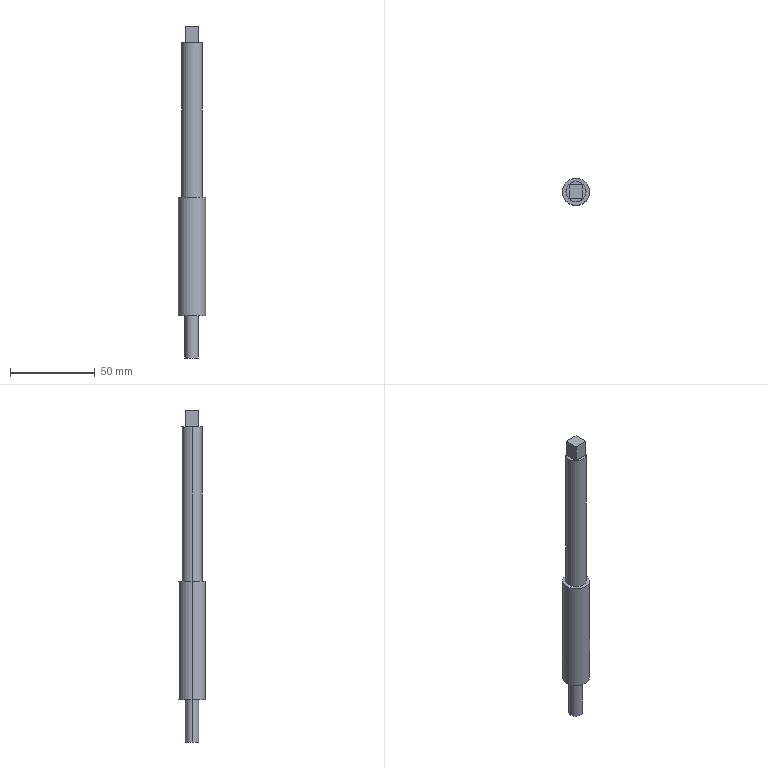Part | SolidWorks | features ICE 3, Extrusion 1 | 1 solid | 15 faces | box 16 x 16 x 196 mm | volume 26092 mm3 | plane 9 | cylinder 6 | commonest cylinder face diameters 8 x2 11.9 x2 16 x2
STEP:
#1=CARTESIAN_POINT('',(-4.225,0.,-95.));
#2=VERTEX_POINT('',#1);
#3=CARTESIAN_POINT('',(3.775,0.,-95.));
#4=VERTEX_POINT('',#3);
#5=CARTESIAN_POINT('',(-0.2246,0.,-95.));
#6=DIRECTION('',(0.,0.,-1.));
#7=DIRECTION('',(-1.,0.,0.));
#8=AXIS2_PLACEMENT_3D('',#5,#6,#7);
#9=CIRCLE('',#8,4.);
#10=EDGE_CURVE('',#2,#4,#9,.T.);
#11=ORIENTED_EDGE('',*,*,#10,.F.);
#12=CARTESIAN_POINT('',(-4.225,0.,-70.));
#13=VERTEX_POINT('',#12);
#14=CARTESIAN_POINT('',(-4.225,0.,-95.));
#15=DIRECTION('',(0.,0.,1.));
#16=VECTOR('',#15,1000.);
#17=LINE('',#14,#16);
#18=EDGE_CURVE('',#2,#13,#17,.T.);
#19=ORIENTED_EDGE('',*,*,#18,.T.);
#20=CARTESIAN_POINT('',(3.775,0.,-70.));
#21=VERTEX_POINT('',#20);
#22=CARTESIAN_POINT('',(-0.2246,0.,-70.));
#23=DIRECTION('',(0.,0.,-1.));
#24=DIRECTION('',(-1.,0.,0.));
#25=AXIS2_PLACEMENT_3D('',#22,#23,#24);
#26=CIRCLE('',#25,4.);
#27=EDGE_CURVE('',#13,#21,#26,.T.);
#28=ORIENTED_EDGE('',*,*,#27,.T.);
#29=CARTESIAN_POINT('',(3.775,0.,-95.));
#30=DIRECTION('',(0.,0.,1.));
#31=VECTOR('',#30,1000.);
#32=LINE('',#29,#31);
#33=EDGE_CURVE('',#4,#21,#32,.T.);
#34=ORIENTED_EDGE('',*,*,#33,.F.);
#35=EDGE_LOOP('',(#11,#19,#28,#34));
#36=FACE_OUTER_BOUND('',#35,.T.);
#37=CARTESIAN_POINT('',(-0.2246,0.,-95.));
#38=DIRECTION('',(0.,0.,1.));
#39=DIRECTION('',(1.,0.,0.));
#40=AXIS2_PLACEMENT_3D('',#37,#38,#39);
#41=CYLINDRICAL_SURFACE('',#40,4.);
#42=ADVANCED_FACE('',(#36),#41,.T.);
#43=CARTESIAN_POINT('',(-8.,0.,-70.));
#44=VERTEX_POINT('',#43);
#45=CARTESIAN_POINT('',(8.,0.,-70.));
#46=VERTEX_POINT('',#45);
#47=CARTESIAN_POINT('',(0.,0.,-70.));
#48=DIRECTION('',(0.,0.,-1.));
#49=DIRECTION('',(-1.,0.,0.));
#50=AXIS2_PLACEMENT_3D('',#47,#48,#49);
#51=CIRCLE('',#50,8.);
#52=EDGE_CURVE('',#44,#46,#51,.T.);
#53=ORIENTED_EDGE('',*,*,#52,.F.);
#54=CARTESIAN_POINT('',(-8.,0.,0.));
#55=VERTEX_POINT('',#54);
#56=CARTESIAN_POINT('',(-8.,0.,-70.));
#57=DIRECTION('',(0.,0.,1.));
#58=VECTOR('',#57,1000.);
#59=LINE('',#56,#58);
#60=EDGE_CURVE('',#44,#55,#59,.T.);
#61=ORIENTED_EDGE('',*,*,#60,.T.);
#62=CARTESIAN_POINT('',(8.,0.,0.));
#63=VERTEX_POINT('',#62);
#64=CARTESIAN_POINT('',(0.,0.,0.));
#65=DIRECTION('',(0.,0.,-1.));
#66=DIRECTION('',(-1.,0.,0.));
#67=AXIS2_PLACEMENT_3D('',#64,#65,#66);
#68=CIRCLE('',#67,8.);
#69=EDGE_CURVE('',#55,#63,#68,.T.);
#70=ORIENTED_EDGE('',*,*,#69,.T.);
#71=CARTESIAN_POINT('',(8.,0.,-70.));
#72=DIRECTION('',(0.,0.,1.));
#73=VECTOR('',#72,1000.);
#74=LINE('',#71,#73);
#75=EDGE_CURVE('',#46,#63,#74,.T.);
#76=ORIENTED_EDGE('',*,*,#75,.F.);
#77=EDGE_LOOP('',(#53,#61,#70,#76));
#78=FACE_OUTER_BOUND('',#77,.T.);
#79=CARTESIAN_POINT('',(0.,0.,-70.));
#80=DIRECTION('',(0.,0.,1.));
#81=DIRECTION('',(1.,0.,0.));
#82=AXIS2_PLACEMENT_3D('',#79,#80,#81);
#83=CYLINDRICAL_SURFACE('',#82,8.);
#84=ADVANCED_FACE('',(#78),#83,.T.);
#85=CARTESIAN_POINT('',(5.95,0.,91.));
#86=VERTEX_POINT('',#85);
#87=CARTESIAN_POINT('',(-5.95,0.,91.));
#88=VERTEX_POINT('',#87);
#89=CARTESIAN_POINT('',(0.,0.,91.));
#90=DIRECTION('',(0.,0.,1.));
#91=DIRECTION('',(1.,0.,0.));
#92=AXIS2_PLACEMENT_3D('',#89,#90,#91);
#93=CIRCLE('',#92,5.95);
#94=EDGE_CURVE('',#86,#88,#93,.T.);
#95=ORIENTED_EDGE('',*,*,#94,.F.);
#96=CARTESIAN_POINT('',(5.95,0.,0.));
#97=VERTEX_POINT('',#96);
#98=CARTESIAN_POINT('',(5.95,0.,91.));
#99=DIRECTION('',(0.,0.,-1.));
#100=VECTOR('',#99,1000.);
#101=LINE('',#98,#100);
#102=EDGE_CURVE('',#86,#97,#101,.T.);
#103=ORIENTED_EDGE('',*,*,#102,.T.);
#104=CARTESIAN_POINT('',(-5.95,0.,0.));
#105=VERTEX_POINT('',#104);
#106=CARTESIAN_POINT('',(0.,0.,0.));
#107=DIRECTION('',(0.,0.,-1.));
#108=DIRECTION('',(-1.,0.,0.));
#109=AXIS2_PLACEMENT_3D('',#106,#107,#108);
#110=CIRCLE('',#109,5.95);
#111=EDGE_CURVE('',#105,#97,#110,.T.);
#112=ORIENTED_EDGE('',*,*,#111,.F.);
#113=CARTESIAN_POINT('',(-5.95,0.,91.));
#114=DIRECTION('',(0.,0.,-1.));
#115=VECTOR('',#114,1000.);
#116=LINE('',#113,#115);
#117=EDGE_CURVE('',#88,#105,#116,.T.);
#118=ORIENTED_EDGE('',*,*,#117,.F.);
#119=EDGE_LOOP('',(#95,#103,#112,#118));
#120=FACE_OUTER_BOUND('',#119,.T.);
#121=CARTESIAN_POINT('',(0.,0.,91.));
#122=DIRECTION('',(0.,0.,-1.));
#123=DIRECTION('',(-1.,0.,0.));
#124=AXIS2_PLACEMENT_3D('',#121,#122,#123);
#125=CYLINDRICAL_SURFACE('',#124,5.95);
#126=ADVANCED_FACE('',(#120),#125,.T.);
#127=CARTESIAN_POINT('',(0.,0.,-70.));
#128=DIRECTION('',(0.,0.,-1.));
#129=DIRECTION('',(-1.,0.,0.));
#130=AXIS2_PLACEMENT_3D('',#127,#128,#129);
#131=CIRCLE('',#130,8.);
#132=EDGE_CURVE('',#46,#44,#131,.T.);
#133=ORIENTED_EDGE('',*,*,#132,.T.);
#134=ORIENTED_EDGE('',*,*,#52,.T.);
#135=EDGE_LOOP('',(#133,#134));
#136=FACE_OUTER_BOUND('',#135,.T.);
#137=CARTESIAN_POINT('',(-0.2246,0.,-70.));
#138=DIRECTION('',(0.,0.,-1.));
#139=DIRECTION('',(-1.,0.,0.));
#140=AXIS2_PLACEMENT_3D('',#137,#138,#139);
#141=CIRCLE('',#140,4.);
#142=EDGE_CURVE('',#21,#13,#141,.T.);
#143=ORIENTED_EDGE('',*,*,#142,.F.);
#144=ORIENTED_EDGE('',*,*,#27,.F.);
#145=EDGE_LOOP('',(#143,#144));
#146=FACE_BOUND('',#145,.T.);
#147=CARTESIAN_POINT('',(0.,0.,-70.));
#148=DIRECTION('',(0.,0.,-1.));
#149=DIRECTION('',(-1.,0.,0.));
#150=AXIS2_PLACEMENT_3D('',#147,#148,#149);
#151=PLANE('',#150);
#152=ADVANCED_FACE('',(#136,#146),#151,.T.);
#153=CARTESIAN_POINT('',(0.,0.,91.));
#154=DIRECTION('',(0.,0.,1.));
#155=DIRECTION('',(1.,0.,0.));
#156=AXIS2_PLACEMENT_3D('',#153,#154,#155);
#157=CIRCLE('',#156,5.95);
#158=EDGE_CURVE('',#88,#86,#157,.T.);
#159=ORIENTED_EDGE('',*,*,#158,.T.);
#160=ORIENTED_EDGE('',*,*,#94,.T.);
#161=EDGE_LOOP('',(#159,#160));
#162=FACE_OUTER_BOUND('',#161,.T.);
#163=CARTESIAN_POINT('',(-4.,-4.,91.));
#164=VERTEX_POINT('',#163);
#165=CARTESIAN_POINT('',(4.,-4.,91.));
#166=VERTEX_POINT('',#165);
#167=CARTESIAN_POINT('',(4.,-4.,91.));
#168=DIRECTION('',(1.,0.,0.));
#169=VECTOR('',#168,1000.);
#170=LINE('',#167,#169);
#171=EDGE_CURVE('',#164,#166,#170,.T.);
#172=ORIENTED_EDGE('',*,*,#171,.F.);
#173=CARTESIAN_POINT('',(-4.,4.,91.));
#174=VERTEX_POINT('',#173);
#175=CARTESIAN_POINT('',(-4.,4.,91.));
#176=DIRECTION('',(0.,-1.,0.));
#177=VECTOR('',#176,1000.);
#178=LINE('',#175,#177);
#179=EDGE_CURVE('',#174,#164,#178,.T.);
#180=ORIENTED_EDGE('',*,*,#179,.F.);
#181=CARTESIAN_POINT('',(4.,4.,91.));
#182=VERTEX_POINT('',#181);
#183=CARTESIAN_POINT('',(4.,4.,91.));
#184=DIRECTION('',(-1.,0.,0.));
#185=VECTOR('',#184,1000.);
#186=LINE('',#183,#185);
#187=EDGE_CURVE('',#182,#174,#186,.T.);
#188=ORIENTED_EDGE('',*,*,#187,.F.);
#189=CARTESIAN_POINT('',(4.,4.,91.));
#190=DIRECTION('',(0.,1.,0.));
#191=VECTOR('',#190,1000.);
#192=LINE('',#189,#191);
#193=EDGE_CURVE('',#166,#182,#192,.T.);
#194=ORIENTED_EDGE('',*,*,#193,.F.);
#195=EDGE_LOOP('',(#172,#180,#188,#194));
#196=FACE_BOUND('',#195,.T.);
#197=CARTESIAN_POINT('',(0.,0.,91.));
#198=DIRECTION('',(0.,0.,1.));
#199=DIRECTION('',(1.,0.,0.));
#200=AXIS2_PLACEMENT_3D('',#197,#198,#199);
#201=PLANE('',#200);
#202=ADVANCED_FACE('',(#162,#196),#201,.T.);
#203=ORIENTED_EDGE('',*,*,#102,.F.);
#204=ORIENTED_EDGE('',*,*,#158,.F.);
#205=ORIENTED_EDGE('',*,*,#117,.T.);
#206=CARTESIAN_POINT('',(0.,0.,0.));
#207=DIRECTION('',(0.,0.,-1.));
#208=DIRECTION('',(-1.,0.,0.));
#209=AXIS2_PLACEMENT_3D('',#206,#207,#208);
#210=CIRCLE('',#209,5.95);
#211=EDGE_CURVE('',#97,#105,#210,.T.);
#212=ORIENTED_EDGE('',*,*,#211,.F.);
#213=EDGE_LOOP('',(#203,#204,#205,#212));
#214=FACE_OUTER_BOUND('',#213,.T.);
#215=CARTESIAN_POINT('',(0.,0.,91.));
#216=DIRECTION('',(0.,0.,-1.));
#217=DIRECTION('',(-1.,0.,0.));
#218=AXIS2_PLACEMENT_3D('',#215,#216,#217);
#219=CYLINDRICAL_SURFACE('',#218,5.95);
#220=ADVANCED_FACE('',(#214),#219,.T.);
#221=ORIENTED_EDGE('',*,*,#179,.T.);
#222=CARTESIAN_POINT('',(-4.,-4.,101.));
#223=VERTEX_POINT('',#222);
#224=CARTESIAN_POINT('',(-4.,-4.,101.));
#225=DIRECTION('',(0.,0.,-1.));
#226=VECTOR('',#225,1000.);
#227=LINE('',#224,#226);
#228=EDGE_CURVE('',#223,#164,#227,.T.);
#229=ORIENTED_EDGE('',*,*,#228,.F.);
#230=CARTESIAN_POINT('',(-4.,4.,101.));
#231=VERTEX_POINT('',#230);
#232=CARTESIAN_POINT('',(-4.,4.,101.));
#233=DIRECTION('',(0.,-1.,0.));
#234=VECTOR('',#233,1000.);
#235=LINE('',#232,#234);
#236=EDGE_CURVE('',#231,#223,#235,.T.);
#237=ORIENTED_EDGE('',*,*,#236,.F.);
#238=CARTESIAN_POINT('',(-4.,4.,101.));
#239=DIRECTION('',(0.,0.,-1.));
#240=VECTOR('',#239,1000.);
#241=LINE('',#238,#240);
#242=EDGE_CURVE('',#231,#174,#241,.T.);
#243=ORIENTED_EDGE('',*,*,#242,.T.);
#244=EDGE_LOOP('',(#221,#229,#237,#243));
#245=FACE_OUTER_BOUND('',#244,.T.);
#246=CARTESIAN_POINT('',(-4.,4.,101.));
#247=DIRECTION('',(1.,0.,0.));
#248=DIRECTION('',(0.,1.,0.));
#249=AXIS2_PLACEMENT_3D('',#246,#247,#248);
#250=PLANE('',#249);
#251=ADVANCED_FACE('',(#245),#250,.F.);
#252=ORIENTED_EDGE('',*,*,#171,.T.);
#253=CARTESIAN_POINT('',(4.,-4.,101.));
#254=VERTEX_POINT('',#253);
#255=CARTESIAN_POINT('',(4.,-4.,101.));
#256=DIRECTION('',(0.,0.,-1.));
#257=VECTOR('',#256,1000.);
#258=LINE('',#255,#257);
#259=EDGE_CURVE('',#254,#166,#258,.T.);
#260=ORIENTED_EDGE('',*,*,#259,.F.);
#261=CARTESIAN_POINT('',(4.,-4.,101.));
#262=DIRECTION('',(1.,0.,0.));
#263=VECTOR('',#262,1000.);
#264=LINE('',#261,#263);
#265=EDGE_CURVE('',#223,#254,#264,.T.);
#266=ORIENTED_EDGE('',*,*,#265,.F.);
#267=ORIENTED_EDGE('',*,*,#228,.T.);
#268=EDGE_LOOP('',(#252,#260,#266,#267));
#269=FACE_OUTER_BOUND('',#268,.T.);
#270=CARTESIAN_POINT('',(4.,-4.,101.));
#271=DIRECTION('',(0.,1.,0.));
#272=DIRECTION('',(-1.,0.,0.));
#273=AXIS2_PLACEMENT_3D('',#270,#271,#272);
#274=PLANE('',#273);
#275=ADVANCED_FACE('',(#269),#274,.F.);
#276=ORIENTED_EDGE('',*,*,#193,.T.);
#277=CARTESIAN_POINT('',(4.,4.,101.));
#278=VERTEX_POINT('',#277);
#279=CARTESIAN_POINT('',(4.,4.,101.));
#280=DIRECTION('',(0.,0.,-1.));
#281=VECTOR('',#280,1000.);
#282=LINE('',#279,#281);
#283=EDGE_CURVE('',#278,#182,#282,.T.);
#284=ORIENTED_EDGE('',*,*,#283,.F.);
#285=CARTESIAN_POINT('',(4.,4.,101.));
#286=DIRECTION('',(0.,1.,0.));
#287=VECTOR('',#286,1000.);
#288=LINE('',#285,#287);
#289=EDGE_CURVE('',#254,#278,#288,.T.);
#290=ORIENTED_EDGE('',*,*,#289,.F.);
#291=ORIENTED_EDGE('',*,*,#259,.T.);
#292=EDGE_LOOP('',(#276,#284,#290,#291));
#293=FACE_OUTER_BOUND('',#292,.T.);
#294=CARTESIAN_POINT('',(4.,4.,101.));
#295=DIRECTION('',(-1.,0.,0.));
#296=DIRECTION('',(0.,-1.,0.));
#297=AXIS2_PLACEMENT_3D('',#294,#295,#296);
#298=PLANE('',#297);
#299=ADVANCED_FACE('',(#293),#298,.F.);
#300=ORIENTED_EDGE('',*,*,#187,.T.);
#301=ORIENTED_EDGE('',*,*,#242,.F.);
#302=CARTESIAN_POINT('',(4.,4.,101.));
#303=DIRECTION('',(-1.,0.,0.));
#304=VECTOR('',#303,1000.);
#305=LINE('',#302,#304);
#306=EDGE_CURVE('',#278,#231,#305,.T.);
#307=ORIENTED_EDGE('',*,*,#306,.F.);
#308=ORIENTED_EDGE('',*,*,#283,.T.);
#309=EDGE_LOOP('',(#300,#301,#307,#308));
#310=FACE_OUTER_BOUND('',#309,.T.);
#311=CARTESIAN_POINT('',(4.,4.,101.));
#312=DIRECTION('',(0.,-1.,0.));
#313=DIRECTION('',(0.,0.,-1.));
#314=AXIS2_PLACEMENT_3D('',#311,#312,#313);
#315=PLANE('',#314);
#316=ADVANCED_FACE('',(#310),#315,.F.);
#317=ORIENTED_EDGE('',*,*,#236,.T.);
#318=ORIENTED_EDGE('',*,*,#265,.T.);
#319=ORIENTED_EDGE('',*,*,#289,.T.);
#320=ORIENTED_EDGE('',*,*,#306,.T.);
#321=EDGE_LOOP('',(#317,#318,#319,#320));
#322=FACE_OUTER_BOUND('',#321,.T.);
#323=CARTESIAN_POINT('',(0.,0.,101.));
#324=DIRECTION('',(0.,0.,-1.));
#325=DIRECTION('',(-1.,0.,0.));
#326=AXIS2_PLACEMENT_3D('',#323,#324,#325);
#327=PLANE('',#326);
#328=ADVANCED_FACE('',(#322),#327,.F.);
#329=CARTESIAN_POINT('',(0.,0.,0.));
#330=DIRECTION('',(0.,0.,-1.));
#331=DIRECTION('',(-1.,0.,0.));
#332=AXIS2_PLACEMENT_3D('',#329,#330,#331);
#333=CIRCLE('',#332,8.);
#334=EDGE_CURVE('',#63,#55,#333,.T.);
#335=ORIENTED_EDGE('',*,*,#334,.F.);
#336=ORIENTED_EDGE('',*,*,#69,.F.);
#337=EDGE_LOOP('',(#335,#336));
#338=FACE_OUTER_BOUND('',#337,.T.);
#339=ORIENTED_EDGE('',*,*,#111,.T.);
#340=ORIENTED_EDGE('',*,*,#211,.T.);
#341=EDGE_LOOP('',(#339,#340));
#342=FACE_BOUND('',#341,.T.);
#343=CARTESIAN_POINT('',(0.,0.,0.));
#344=DIRECTION('',(0.,0.,-1.));
#345=DIRECTION('',(-1.,0.,0.));
#346=AXIS2_PLACEMENT_3D('',#343,#344,#345);
#347=PLANE('',#346);
#348=ADVANCED_FACE('',(#338,#342),#347,.F.);
#349=ORIENTED_EDGE('',*,*,#60,.F.);
#350=ORIENTED_EDGE('',*,*,#132,.F.);
#351=ORIENTED_EDGE('',*,*,#75,.T.);
#352=ORIENTED_EDGE('',*,*,#334,.T.);
#353=EDGE_LOOP('',(#349,#350,#351,#352));
#354=FACE_OUTER_BOUND('',#353,.T.);
#355=CARTESIAN_POINT('',(0.,0.,-70.));
#356=DIRECTION('',(0.,0.,1.));
#357=DIRECTION('',(1.,0.,0.));
#358=AXIS2_PLACEMENT_3D('',#355,#356,#357);
#359=CYLINDRICAL_SURFACE('',#358,8.);
#360=ADVANCED_FACE('',(#354),#359,.T.);
#361=ORIENTED_EDGE('',*,*,#18,.F.);
#362=CARTESIAN_POINT('',(-0.2246,0.,-95.));
#363=DIRECTION('',(0.,0.,-1.));
#364=DIRECTION('',(-1.,0.,0.));
#365=AXIS2_PLACEMENT_3D('',#362,#363,#364);
#366=CIRCLE('',#365,4.);
#367=EDGE_CURVE('',#4,#2,#366,.T.);
#368=ORIENTED_EDGE('',*,*,#367,.F.);
#369=ORIENTED_EDGE('',*,*,#33,.T.);
#370=ORIENTED_EDGE('',*,*,#142,.T.);
#371=EDGE_LOOP('',(#361,#368,#369,#370));
#372=FACE_OUTER_BOUND('',#371,.T.);
#373=CARTESIAN_POINT('',(-0.2246,0.,-95.));
#374=DIRECTION('',(0.,0.,1.));
#375=DIRECTION('',(1.,0.,0.));
#376=AXIS2_PLACEMENT_3D('',#373,#374,#375);
#377=CYLINDRICAL_SURFACE('',#376,4.);
#378=ADVANCED_FACE('',(#372),#377,.T.);
#379=ORIENTED_EDGE('',*,*,#367,.T.);
#380=ORIENTED_EDGE('',*,*,#10,.T.);
#381=EDGE_LOOP('',(#379,#380));
#382=FACE_OUTER_BOUND('',#381,.T.);
#383=CARTESIAN_POINT('',(-0.2246,0.,-95.));
#384=DIRECTION('',(0.,0.,-1.));
#385=DIRECTION('',(-1.,0.,0.));
#386=AXIS2_PLACEMENT_3D('',#383,#384,#385);
#387=PLANE('',#386);
#388=ADVANCED_FACE('',(#382),#387,.T.);
#389=CLOSED_SHELL('',(#42,#84,#126,#152,#202,#220,#251,#275,#299,#316,#328,#348,#360,#378,#388));
#390=MANIFOLD_SOLID_BREP('',#389);
#391=CARTESIAN_POINT('',(0.,0.,0.));
#392=DIRECTION('',(0.,0.,1.));
#393=DIRECTION('',(1.,0.,0.));
#394=AXIS2_PLACEMENT_3D('',#391,#392,#393);
#395=(LENGTH_UNIT()NAMED_UNIT(*)SI_UNIT(.MILLI.,.METRE.));
#396=UNCERTAINTY_MEASURE_WITH_UNIT(LENGTH_MEASURE(0.00001),#395,'','');
#397=(NAMED_UNIT(*)PLANE_ANGLE_UNIT()SI_UNIT($,.RADIAN.));
#398=(NAMED_UNIT(*)SI_UNIT($,.STERADIAN.)SOLID_ANGLE_UNIT());
#399=(GEOMETRIC_REPRESENTATION_CONTEXT(3)GLOBAL_UNCERTAINTY_ASSIGNED_CONTEXT((#396))GLOBAL_UNIT_ASSIGNED_CONTEXT((#395,#397,#398))REPRESENTATION_CONTEXT('',''));
#400=ADVANCED_BREP_SHAPE_REPRESENTATION('',(#390,#394),#399);